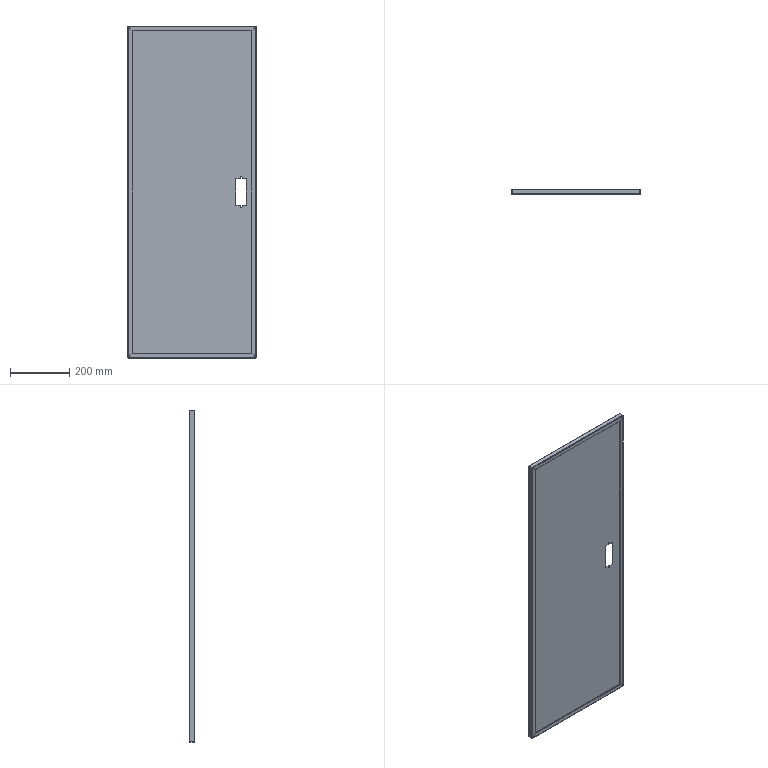Part | 1 solid | 83 faces | box 435 x 18 x 1121 mm | volume 858873 mm3 | plane 48 | cylinder 19 | spline 16 | commonest cylinder face diameters 1.473 x8 4.473 x8 7 x3